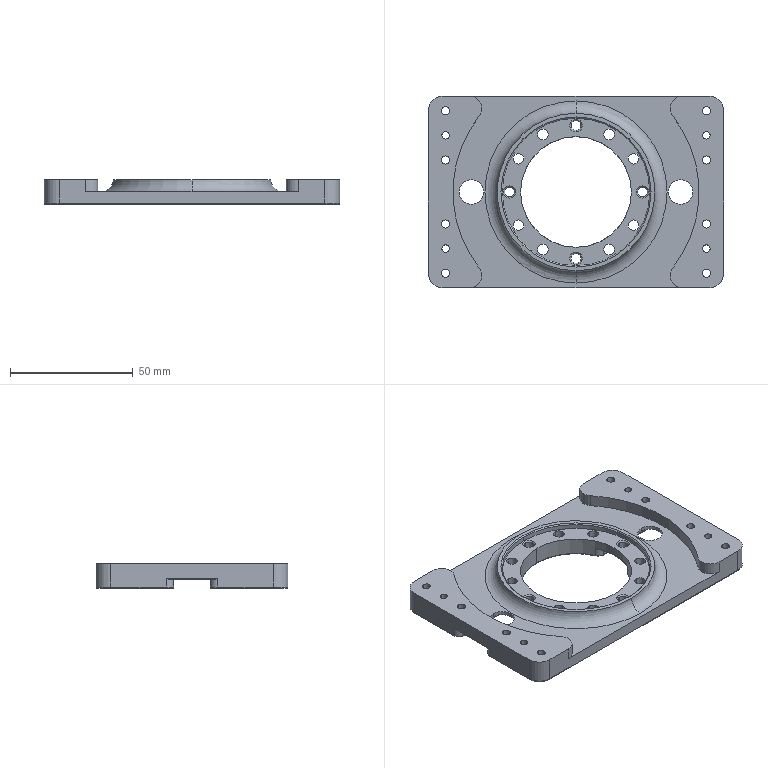NC program | NX | posted with a generic post | part box 120 x 78 x 10 mm
Lines 35 to 888 of 8419:
(ADAPTIVE_MILLING_COPY_1 , TOOL : D10)
N68 T15 M6
N70 G54
N72 G17 G0 G90 X-29.216 Y42.583 B0. C0. S9500 M3
N74 G43 Z30. H15
N76 Z3.
N78 G94 G3 X-29.216 Y42.583 Z2.506 I1.305 J-4.307 F1000.
N80 X-29.216 Y42.583 Z2.013 I1.305 J-4.307
N82 X-29.216 Y42.583 Z1.519 I1.305 J-4.307
N84 X-29.216 Y42.583 Z1.026 I1.305 J-4.307
N86 X-29.216 Y42.583 Z0.532 I1.305 J-4.307
N88 X-29.216 Y42.583 Z0.039 I1.305 J-4.307
N90 X-29.216 Y42.583 Z-0.455 I1.305 J-4.307
N92 X-29.216 Y42.583 Z-0.948 I1.305 J-4.307
N94 X-29.216 Y42.583 Z-1.442 I1.305 J-4.307
N96 X-29.216 Y42.583 Z-1.935 I1.305 J-4.307
N98 X-29.216 Y42.583 Z-2.429 I1.305 J-4.307
N100 X-29.216 Y42.583 Z-2.922 I1.305 J-4.307
N102 X-29.216 Y42.583 Z-3.416 I1.305 J-4.307
N104 X-29.216 Y42.583 Z-3.909 I1.305 J-4.307
N106 X-29.216 Y42.583 Z-4.403 I1.305 J-4.307
N108 X-23.412 Y38.276 Z-4.75 R-4.5
N110 X-24.233 Y35.67 R-4.501 F3000.
N112 X-28.904 Y43.148 R4.673
N114 X-24.107 Y35.033 R-4.978
N116 X-29.565 Y43.485 R5.194
N118 X-24.488 Y33.987 R-5.474
N120 X-22.23 Y38.968 R5.736
N122 X-26.259 Y44. R5.522
N124 X-29.504 Y43.925 R23.784
N126 X-33.902 Y37.98 R5.67
N128 X-33.017 Y35.334 R42.36
N130 X-25.859 Y32.634 R5.739
N132 G2 X-23.479 Y34.38 R62.429
N134 G3 X-23.21 Y42.728 R5.954
N136 X-24.77 Y43.953 R4.725
N138 X-26.263 Y44. R8.377
N140 G1 X-28.759
N142 G3 X-30.982 Y43.785 R5.996
N144 X-34.405 Y39.201 R5.651
N146 X-33.91 Y38.004 R3.106
N148 G1 X-33.87 Y37.886
N150 G3 X-31.896 Y37.646 R1.101
N152 G1 X-28.953 Y42.313
N154 G3 X-29.884 Y44. R1.102
N156 X-33.692 Y42.286 R4.141
N158 X-34.785 Y39.935 R4.907
N160 G1 X-34.689 Y39.448
N162 X-34.269 Y38.68
N164 G3 X-32.399 Y38.583 R1.102
N166 G1 X-29.853 Y42.276
N168 G3 X-30.759 Y44. R1.101
N170 X-34.15 Y42.492 R3.819
N172 X-35.125 Y40.375 R3.599
N174 X-34.774 Y39.604 R1.466
N176 G1 X-34.654 Y39.385
N178 G3 X-32.801 Y39.264 R1.102
N180 G1 X-30.62 Y42.252
N182 G3 X-31.509 Y44. R1.101
N184 X-34.832 Y42.382 R3.64
N186 X-35.433 Y40.652 R2.554
N188 X-34.862 Y39.726 R2.225
N190 X-33.128 Y39.755 R1.103
N192 G1 X-31.256 Y42.238
N194 G3 X-32.134 Y44. R1.101
N196 X-35.752 Y41.266 R3.309
N198 X-35.244 Y40.198 R1.572
N200 X-33.507 Y40.231 R1.103
N202 G1 X-32.003 Y42.241
N204 G3 X-32.884 Y44. R1.101
N206 X-36.031 Y41.587 R2.885
N208 X-35.525 Y40.547 R1.585
N210 X-33.8 Y40.565 R1.103
N212 G1 X-32.514 Y42.227
N214 G3 X-33.384 Y44. R1.101
N216 X-36.282 Y41.996 R2.631
N218 X-35.832 Y40.927 R1.303
N220 X-34.098 Y40.955 R1.103
N222 G1 X-33.131 Y42.237
N224 G3 X-34.009 Y44. R1.101
N226 X-36.533 Y42.113 R2.243
N228 X-35.977 Y41.092 R1.23
N230 X-34.386 Y41.255 R1.104
N232 G1 X-33.954 Y41.808
N234 X-33.541 Y42.376
N236 G3 X-34.509 Y44. R1.102
N238 X-36.761 Y42.197 R1.959
N240 X-36.163 Y41.253 R1.343
N242 X-33.477 Y42.652 R1.627
N244 X-35.009 Y44. R1.549
N246 X-36.951 Y42.244 R1.668
N248 X-36.37 Y41.432 R1.432
N250 X-34.796 Y43.876 R-1.469
N252 G1 X-35.084 Y43.965
N254 X-35.384 Y44.
N256 G3 X-37.134 Y42.387 R1.49
N258 X-36.65 Y41.673 R1.326
N260 X-35.371 Y43.942 R-1.33
N262 G1 X-35.563 Y43.981
N264 X-35.759 Y44.
N266 G3 X-37.254 Y42.381 R1.299
N268 X-36.805 Y41.807 R1.541
N270 X-34.871 Y42.896 R1.185
N272 X-36.134 Y44. R1.28
N274 X-36.954 Y41.935 R1.14
N276 X-35.171 Y42.832 R1.085
N278 X-36.384 Y44. R1.218
N280 X-37.089 Y42.051 R1.073
N282 G1 X-35.91 Y41.024
N284 X-34.774 Y39.604
N286 X-33.91 Y38.004
N288 X-33.345 Y36.276
N290 G3 X-30.887 Y32.471 R4.45
N292 X-26.905 Y31.809 R5.657
N294 X-25.718 Y32.727 R7.011
N296 X-26.059 Y34.611 R1.102
N298 G1 X-31.77 Y36.603
N300 G3 X-33.222 Y35.41 R1.102
N302 X-31.163 Y32.059 R4.006
N304 X-27.713 Y31.192 R5.311
N306 X-26.602 Y31.991 R3.861
N308 X-26.912 Y33.864 R1.102
N310 G1 X-31.61 Y35.664
N312 G3 X-33.101 Y34.559 R1.102
N314 X-31.961 Y32.097 R3.055
N316 X-28.454 Y30.672 R5.173
N318 X-27.959 Y30.862 R4.213
N320 G1 X-27.287 Y31.422
N322 G3 X-27.512 Y33.258 R1.102
N324 G1 X-31.529 Y35.196
N326 G3 X-33.106 Y34.248 R1.102
N328 X-31.927 Y31.494 R3.116
N330 X-28.881 Y30.25 R4.319
N332 X-28.072 Y30.768 R1.522
N334 G1 X-27.88 Y30.928
N336 G3 X-28.045 Y32.733 R1.102
N338 G1 X-31.487 Y34.665
N340 G3 X-33.125 Y33.748 R1.102
N342 X-31.896 Y30.892 R3.172
N344 X-29.292 Y29.854 R3.731
N346 X-28.289 Y30.554 R1.904
N348 X-28.481 Y32.262 R1.103
N350 G1 X-31.459 Y34.137
N352 G3 X-33.144 Y33.249 R1.102
N354 X-31.761 Y30.224 R3.197
N356 X-29.565 Y29.502 R2.968
N358 X-28.667 Y30.175 R2.079
N360 X-28.858 Y31.882 R1.103
N362 G1 X-31.485 Y33.541
N364 G3 X-33.163 Y32.752 R1.102
N366 X-32.408 Y30.263 R2.636
N368 X-29.997 Y29.139 R3.094
N370 X-29.091 Y29.75 R1.694
N372 X-29.226 Y31.419 R1.103
N374 G1 X-31.512 Y33.068
N376 G3 X-33.229 Y32.414 R1.102
N378 X-32.48 Y29.785 R2.614
N380 X-30.268 Y28.824 R2.713
N382 X-29.424 Y29.416 R1.751
N384 X-29.518 Y31.054 R1.103
N386 G1 X-31.552 Y32.671
N388 G3 X-33.31 Y32.047 R1.102
N390 X-32.356 Y29.15 R2.639
N392 X-30.524 Y28.527 R2.255
N394 X-29.73 Y29.11 R1.862
N396 X-29.831 Y30.753 R1.103
N398 G1 X-31.667 Y32.188
N400 G3 X-33.418 Y31.559 R1.102
N402 X-32.391 Y28.703 R2.551
N404 X-30.762 Y28.252 R1.928
N406 X-30.023 Y28.817 R2.004
N408 X-30.141 Y30.473 R1.103
N410 G1 X-31.792 Y31.713
N412 G3 X-33.526 Y31.071 R1.102
N414 X-32.839 Y28.626 R2.276
N416 X-31.041 Y27.975 R1.936
N418 X-30.297 Y28.542 R1.994
N420 X-30.406 Y30.191 R1.103
N422 G1 X-31.893 Y31.331
N424 G3 X-33.576 Y30.884 R1.103
N426 X-33.225 Y28.559 R2.073
N428 X-31.393 Y27.685 R2.031
N430 X-30.615 Y28.223 R1.624
N432 X-30.683 Y29.839 R1.104
N434 G1 X-31.996 Y30.952
N436 G3 X-33.722 Y30.538 R1.103
N438 X-33.185 Y28.035 R2.108
N440 X-31.491 Y27.463 R1.759
N442 X-30.825 Y28.009 R1.548
N444 X-30.939 Y29.531 R1.104
N446 G1 X-32.119 Y30.587
N448 G3 X-33.867 Y30.192 R1.102
N450 X-33.298 Y27.705 R2.059
N452 X-31.584 Y27.258 R1.615
N454 X-31.021 Y27.773 R1.922
N456 X-31.162 Y29.318 R1.104
N458 G1 X-31.788 Y29.851
N460 X-32.43 Y30.364
N462 G3 X-34.012 Y29.847 R1.103
N464 X-33.298 Y27.303 R2.026
N466 X-31.57 Y27.147 R1.399
N468 G1 X-31.465 Y27.237
N470 X-31.226 Y27.526
N472 G3 X-31.318 Y29.028 R1.104
N474 G1 X-31.889 Y29.575
N476 X-32.477 Y30.101
N478 G3 X-34.108 Y29.616 R1.103
N480 X-33.504 Y27.077 R1.979
N482 X-31.78 Y26.897 R1.387
N484 G1 X-31.685 Y26.977
N486 X-31.666 Y26.994
N488 X-31.427 Y27.283
N490 G3 X-31.588 Y28.845 R1.104
N492 G1 X-32.152 Y29.301
N494 X-32.731 Y29.738
N496 G3 X-34.243 Y29.294 R1.104
N498 X-33.985 Y27.134 R1.759
N500 X-32.218 Y26.517 R1.589
N502 X-31.622 Y27.048 R1.784
N504 X-31.79 Y28.616 R1.104
N506 G1 X-32.341 Y29.054
N508 X-32.908 Y29.472
N510 G3 X-34.356 Y29.106 R1.106
N512 X-34.176 Y26.916 R1.749
N514 X-32.418 Y26.281 R1.581
N516 X-31.814 Y26.816 R1.765
N518 X-31.946 Y28.353 R1.104
N520 G1 X-32.462 Y28.801
N522 X-32.992 Y29.232
N524 G3 X-34.492 Y28.896 R1.104
N526 X-34.287 Y26.608 R1.768
N528 X-32.617 Y26.049 R1.538
N530 X-32.002 Y26.589 R1.737
N532 X-32.101 Y28.097 R1.104
N534 G1 X-32.59 Y28.557
N536 X-33.094 Y29.001
N538 G3 X-34.629 Y28.687 R1.104
N540 X-34.391 Y26.306 R1.771
N542 X-32.702 Y25.872 R1.442
N544 X-32.188 Y26.365 R2.331
N546 X-32.345 Y27.923 R1.104
N548 G1 X-32.846 Y28.331
N550 X-33.359 Y28.724
N552 G3 X-34.833 Y28.372 R1.104
N554 X-34.581 Y26.094 R1.741
N556 X-32.896 Y25.643 R1.44
N558 X-32.371 Y26.144 R2.289
N560 X-32.498 Y27.677 R1.104
N562 G1 X-32.975 Y28.094
N564 X-33.465 Y28.496
N566 G3 X-34.969 Y28.163 R1.104
N568 X-34.766 Y25.886 R1.715
N570 X-33.087 Y25.419 R1.432
N572 X-32.552 Y25.926 R2.257
N574 X-32.751 Y27.517 R1.104
N576 G1 X-33.247 Y27.883
N578 X-33.756 Y28.231
N580 G3 X-35.174 Y27.848 R1.106
N582 X-34.922 Y25.651 R1.697
N584 X-33.239 Y25.217 R1.406
N586 X-32.737 Y25.702 R2.399
N588 X-32.868 Y27.239 R1.104
N590 G1 X-33.325 Y27.637
N592 X-33.798 Y28.016
N594 G3 X-35.261 Y27.716 R1.106
N596 X-35.107 Y25.446 R1.675
N598 X-33.321 Y25.061 R1.374
N600 G1 X-32.914 Y25.489
N602 G3 X-33.022 Y27.006 R1.104
N604 G1 X-33.458 Y27.405
N606 X-33.907 Y27.79
N608 G3 X-35.406 Y27.512 R1.104
N610 X-35.291 Y25.241 R1.673
N612 X-33.616 Y24.773 R1.41
N614 X-33.09 Y25.276 R2.26
N616 X-33.282 Y26.862 R1.104
N618 G1 X-33.747 Y27.211
N620 X-34.224 Y27.543
N622 G3 X-35.625 Y27.208 R1.106
N624 X-35.468 Y25.036 R1.655
N626 X-33.797 Y24.539 R1.436
N628 X-33.279 Y25.045 R1.538
N630 X-33.404 Y26.438 R1.106
N632 G1 X-33.808 Y26.851
N634 X-34.225 Y27.25
N636 G3 X-35.771 Y27.005 R1.104
N638 X-35.565 Y24.741 R1.665
N640 X-33.871 Y24.359 R1.397
N642 X-33.364 Y24.921 R1.951
N644 X-33.572 Y26.39 R1.106
N646 G1 X-34.014 Y26.76
N648 X-34.47 Y27.112
N650 G3 X-35.916 Y26.801 R1.106
N652 X-35.742 Y24.537 R1.657
N654 X-33.946 Y24.188 R1.384
N656 X-33.515 Y24.698 R2.672
N658 X-33.708 Y26.154 R1.106
N660 G1 X-34.146 Y26.536
N662 X-34.599 Y26.899
N664 G3 X-36.062 Y26.598 R1.106
N666 X-35.916 Y24.333 R1.651
N668 X-34.124 Y23.947 R1.403
N670 X-33.666 Y24.478 R2.38
N672 X-33.955 Y26.008 R1.104
N674 G1 X-34.429 Y26.335
N676 X-34.914 Y26.646
N678 G3 X-36.28 Y26.293 R1.106
N680 X-36.094 Y24.128 R1.639
N682 X-34.413 Y23.642 R1.469
N684 X-33.815 Y24.26 R1.675
N686 X-34.09 Y25.78 R1.104
N688 G1 X-34.563 Y26.116
N690 X-35.047 Y26.436
N692 G3 X-36.426 Y26.09 R1.106
N694 X-36.27 Y23.923 R1.634
N696 X-34.595 Y23.402 R1.495
N698 X-33.978 Y24.022 R1.593
N700 X-34.219 Y25.517 R1.104
N702 G1 X-34.682 Y25.875
N704 X-35.158 Y26.216
N706 G3 X-36.572 Y25.887 R1.106
N708 X-36.362 Y23.625 R1.662
N710 X-34.667 Y23.216 R1.432
N712 X-34.135 Y23.792 R1.829
N714 X-34.352 Y25.269 R1.106
N716 G1 X-34.809 Y25.643
N718 X-35.28 Y26.
N720 G3 X-36.717 Y25.684 R1.106
N722 X-36.542 Y23.419 R1.661
N724 X-34.745 Y23.038 R1.415
N726 X-34.286 Y23.57 R2.373
N728 X-34.488 Y25.034 R1.106
N730 G1 X-34.942 Y25.42
N732 X-35.41 Y25.787
N734 G3 X-36.863 Y25.481 R1.106
N736 X-36.721 Y23.214 R1.661
N738 X-34.928 Y22.793 R1.438
N740 X-34.437 Y23.35 R2.218
N742 X-34.733 Y24.885 R1.104
N744 G1 X-35.223 Y25.216
N746 X-35.723 Y25.532
N748 G3 X-37.082 Y25.176 R1.106
N750 X-36.983 Y23.103 R1.623
N752 X-35.224 Y22.487 R1.545
N754 X-34.601 Y23.11 R1.581
N756 X-34.861 Y24.619 R1.104
N758 G1 X-35.341 Y24.974
N760 X-35.832 Y25.311
N762 G3 X-37.227 Y24.973 R1.106
N764 X-37.081 Y22.802 R1.647
N766 X-35.41 Y22.245 R1.54
N768 X-34.758 Y22.881 R1.535
N770 X-34.994 Y24.372 R1.104
N772 G1 X-35.468 Y24.743
N774 X-35.955 Y25.096
N776 G3 X-37.373 Y24.77 R1.106
N778 X-37.228 Y22.559 R1.658
N780 X-35.552 Y22.021 R1.529
N782 X-34.916 Y22.649 R1.558
N784 X-35.169 Y24.154 R1.104
N786 G1 X-35.651 Y24.516
N788 X-36.146 Y24.861
N790 G3 X-37.547 Y24.526 R1.106
N792 X-37.147 Y22.108 R1.736
N794 X-35.279 Y22.118 R1.296
N796 G1 X-35.067 Y22.428
N798 G3 X-35.301 Y23.917 R1.104
N800 G1 X-35.767 Y24.284
N802 X-36.246 Y24.635
N804 G3 X-37.726 Y24.232 R1.104
N806 X-37.317 Y21.892 R1.704
N808 X-35.509 Y21.81 R1.313
N810 G1 X-35.425 Y21.903
N812 X-35.211 Y22.217
N814 G3 X-35.552 Y23.781 R1.104
N816 G1 X-36.05 Y24.084
N818 X-36.557 Y24.37
N820 G3 X-37.917 Y23.909 R1.106
N822 X-37.478 Y21.673 R1.685
N824 X-35.669 Y21.564 R1.324
N826 G1 X-35.584 Y21.656
N828 X-35.513 Y21.749
N830 X-35.448 Y21.866
N832 X-35.423 Y21.908
N834 G3 X-35.632 Y23.312 R1.106
N836 G1 X-36.065 Y23.697
N838 X-36.511 Y24.066
N840 G3 X-38.044 Y23.693 R1.104
N842 X-37.643 Y21.454 R1.672
N844 X-35.826 Y21.304 R1.357
N846 X-35.467 Y21.833 R3.346
N848 X-35.801 Y23.27 R1.106
N850 G1 X-36.27 Y23.601
N852 X-36.752 Y23.913
N854 G3 X-38.171 Y23.478 R1.106
N856 X-37.802 Y21.235 R1.669
N858 X-36.08 Y20.971 R1.424
N860 X-35.597 Y21.598 R1.805
N862 X-35.915 Y23.024 R1.106
N864 G1 X-36.382 Y23.367
N866 X-36.863 Y23.69
N868 G3 X-38.298 Y23.263 R1.106
N870 X-37.861 Y20.939 R1.669
N872 X-36.045 Y20.875 R1.343
N874 G1 X-35.726 Y21.367
N876 G3 X-36.149 Y22.86 R1.104
N878 G1 X-36.648 Y23.144
N880 X-37.157 Y23.412
N882 G3 X-38.488 Y22.94 R1.106
N884 X-38.116 Y20.799 R1.638
N886 X-36.296 Y20.532 R1.429
N888 X-35.856 Y21.132 R2.134
N890 X-36.261 Y22.614 R1.104
N892 G1 X-36.758 Y22.91
N894 X-37.266 Y23.189
N896 G3 X-38.615 Y22.725 R1.106
N898 X-38.277 Y20.579 R1.634
N900 X-36.455 Y20.274 R1.462
N902 X-35.993 Y20.886 R1.903
N904 X-36.368 Y22.35 R1.104
N906 G1 X-36.86 Y22.665
N908 X-37.364 Y22.962
N910 G3 X-38.743 Y22.509 R1.106
N912 X-38.34 Y20.277 R1.647
N914 X-36.614 Y20.015 R1.444
N916 X-36.126 Y20.646 R1.788
N918 X-36.479 Y22.096 R1.106
N920 G1 X-36.968 Y22.426
N922 X-37.469 Y22.737
N924 G3 X-38.87 Y22.294 R1.106
N926 X-38.499 Y20.058 R1.64
N928 X-36.776 Y19.755 R1.467
N930 X-36.257 Y20.411 R1.706
N932 X-36.593 Y21.849 R1.106
N934 G1 X-37.08 Y22.191
N936 X-37.58 Y22.514
N938 G3 X-38.997 Y22.079 R1.106
N940 X-38.656 Y19.836 R1.65
N942 X-36.936 Y19.498 R1.487
N944 X-36.393 Y20.166 R1.634
N946 X-36.817 Y21.66 R1.104
N948 G1 X-37.332 Y21.953
N950 X-37.857 Y22.228
N952 G3 X-39.187 Y21.756 R1.106
N954 X-38.906 Y19.702 R1.615
N956 X-37.101 Y19.238 R1.55
N958 X-36.53 Y19.919 R1.566
N960 X-36.923 Y21.395 R1.104
N962 G1 X-37.433 Y21.707
N964 X-37.954 Y22.001
N966 G3 X-39.314 Y21.54 R1.106
N968 X-38.979 Y19.391 R1.649
N970 X-37.266 Y18.979 R1.549
N972 X-36.664 Y19.678 R1.522
N974 X-37.034 Y21.14 R1.104
N976 G1 X-37.54 Y21.467
N978 X-38.058 Y21.776
N980 G3 X-39.441 Y21.325 R1.106
N982 X-39.059 Y19.096 R1.667
N984 X-37.232 Y18.844 R1.451
N986 X-36.794 Y19.444 R2.174
N988 X-37.203 Y20.93 R1.104
N990 G1 X-37.724 Y21.237
N992 X-38.256 Y21.525
N994 G3 X-39.62 Y21.014 R1.106
N996 X-39.015 Y18.713 R1.72
N998 X-37.201 Y18.758 R1.332
N1000 G1 X-37.116 Y18.865
N1002 X-36.934 Y19.193
N1004 G3 X-37.378 Y20.698 R1.104
N1006 G1 X-37.901 Y20.981
N1008 X-38.434 Y21.244
N1010 G3 X-39.781 Y20.675 R1.106
N1012 X-39.163 Y18.48 R1.695
N1014 X-37.346 Y18.504 R1.339
N1016 G1 X-37.267 Y18.6
N1018 X-37.251 Y18.622
N1020 X-37.069 Y18.95
N1022 G3 X-37.486 Y20.44 R1.104
N1024 G1 X-37.995 Y20.734
N1026 X-38.515 Y21.009
N1028 G3 X-39.889 Y20.45 R1.106
N1030 X-39.307 Y18.25 R1.672
N1032 X-37.578 Y18.161 R1.373
N1034 X-37.232 Y18.655 R3.054
N1036 X-37.566 Y20.092 R1.106
N1038 G1 X-38.04 Y20.425
N1040 X-38.525 Y20.742
N1042 G3 X-39.996 Y20.224 R1.104
N1044 X-39.452 Y18.019 R1.658
N1046 X-37.624 Y17.978 R1.378
N1048 X-37.334 Y18.459 R2.923
N1050 X-37.76 Y19.834 R1.106
N1052 G1 X-38.241 Y20.137
N1054 X-38.732 Y20.424
N1056 G3 X-40.157 Y19.885 R1.104
N1058 X-39.589 Y17.788 R1.638
N1060 X-37.85 Y17.626 R1.447
N1062 X-37.388 Y18.335 R1.69
N1064 X-37.928 Y19.771 R1.104
N1066 G1 X-38.443 Y20.016
N1068 X-38.965 Y20.243
N1070 G3 X-40.265 Y19.66 R1.106
N1072 X-39.625 Y17.483 R1.649
N1074 X-37.802 Y17.524 R1.362
N1076 X-37.5 Y18.078 R3.781
N1078 X-38.01 Y19.499 R1.104
N1080 G1 X-38.522 Y19.763
N1082 X-39.043 Y20.008
N1084 G3 X-40.372 Y19.434 R1.106
N1086 X-39.862 Y17.324 R1.63
N1088 X-38.024 Y17.164 R1.454
N1090 X-37.61 Y17.826 R1.842
N1092 X-38.096 Y19.236 R1.106
N1094 G1 X-38.607 Y19.515
N1096 X-39.128 Y19.775
N1098 G3 X-40.48 Y19.208 R1.106
N1100 X-40.001 Y17.092 R1.626
N1102 X-38.16 Y16.892 R1.484
N1104 X-37.718 Y17.581 R1.737
N1106 X-38.187 Y18.981 R1.106
N1108 G1 X-38.697 Y19.272
N1110 X-39.219 Y19.544
N1112 G3 X-40.587 Y18.982 R1.106
N1114 X-40.042 Y16.782 R1.645
N1116 X-38.203 Y16.7 R1.436
N1118 X-37.824 Y17.339 R2.217
N1120 X-38.403 Y18.793 R1.104
N1122 G1 X-38.941 Y19.024
N1124 X-39.485 Y19.237
N1126 G3 X-40.748 Y18.644 R1.106
N1128 X-40.181 Y16.547 R1.635
N1130 X-38.436 Y16.346 R1.509
N1132 X-37.94 Y17.073 R1.583
N1134 X-38.479 Y18.509 R1.104
N1136 G1 X-39.013 Y18.765
N1138 X-39.555 Y19.001
N1140 G3 X-40.856 Y18.418 R1.106
N1142 X-40.321 Y16.313 R1.632
N1144 X-38.477 Y16.146 R1.485
N1146 X-38.051 Y16.819 R1.792
N1148 X-38.564 Y18.242 R1.104
N1150 G1 X-39.096 Y18.515
N1152 X-39.637 Y18.768
N1154 G3 X-40.963 Y18.192 R1.106
N1156 X-40.458 Y16.08 R1.631
N1158 X-38.613 Y15.873 R1.507
N1160 X-38.159 Y16.574 R1.707
N1162 X-38.654 Y17.988 R1.104
N1164 G1 X-39.186 Y18.272
N1166 X-39.728 Y18.537
N1168 G3 X-41.071 Y17.967 R1.106
N1170 X-40.5 Y15.769 R1.655
N1172 X-38.753 Y15.596 R1.507
N1174 X-38.273 Y16.313 R1.622
N1176 X-38.737 Y17.711 R1.106
N1178 G1 X-39.265 Y18.016
N1180 X-39.805 Y18.301
N1182 G3 X-41.178 Y17.741 R1.106
N1184 X-40.651 Y15.545 R1.653
N1186 X-38.806 Y15.386 R1.483
N1188 X-38.385 Y16.055 R1.81
N1190 X-38.949 Y17.503 R1.104
N1192 G1 X-39.502 Y17.752
N1194 X-40.065 Y17.98
N1196 G3 X-41.372 Y17.298 R1.106
N1198 X-40.574 Y15.157 R1.709
N1200 X-38.757 Y15.298 R1.36
N1202 G1 X-38.683 Y15.4
N1204 X-38.645 Y15.462
N1206 X-38.495 Y15.805
N1208 G3 X-39.035 Y17.242 R1.104
N1210 G1 X-39.578 Y17.502
N1212 X-40.13 Y17.74
N1214 G3 X-41.459 Y17.064 R1.106
N1216 X-40.592 Y14.85 R1.714
N1218 X-38.755 Y15.21 R1.299
N1220 G1 X-38.605 Y15.554
N1222 G3 X-39.12 Y16.978 R1.104
N1224 G1 X-39.645 Y17.244
N1226 X-40.177 Y17.493
N1228 G3 X-41.546 Y16.829 R1.104
N1230 X-40.825 Y14.671 R1.674
N1232 X-39.088 Y14.67 R1.402
N1234 X-38.715 Y15.303 R2.261
N1236 X-39.332 Y16.773 R1.104
N1238 G1 X-39.873 Y16.982
N1240 X-40.421 Y17.172
N1242 G3 X-41.677 Y16.478 R1.106
N1244 X-40.842 Y14.361 R1.674
N1246 X-39.044 Y14.593 R1.324
N1248 G1 X-38.977 Y14.699
N1250 X-38.937 Y14.782
N1252 X-38.928 Y14.81
N1254 X-38.909 Y14.858
N1256 X-38.859 Y14.973
N1258 G3 X-39.362 Y16.391 R1.104
N1260 G1 X-39.869 Y16.656
N1262 X-40.383 Y16.904
N1264 G3 X-41.764 Y16.243 R1.104
N1266 X-40.961 Y14.117 R1.668
N1268 X-39.151 Y14.31 R1.349
N1270 X-38.928 Y14.81 R4.372
N1272 X-39.435 Y16.111 R1.106
N1274 G1 X-39.932 Y16.393
N1276 X-40.438 Y16.658
N1278 G3 X-41.851 Y16.009 R1.104
N1280 X-41.079 Y13.874 R1.652
N1282 X-39.257 Y14.025 R1.376
N1284 X-38.983 Y14.641 R2.591
N1286 X-39.564 Y15.98 R1.106
N1288 G1 X-40.083 Y16.226
N1290 X-40.612 Y16.452
N1292 G3 X-41.938 Y15.775 R1.106
N1294 X-41.089 Y13.568 R1.668
N1296 X-39.29 Y13.838 R1.344
N1298 G1 X-39.064 Y14.392
N1300 G3 X-39.765 Y15.778 R1.104
N1302 G1 X-40.307 Y15.96
N1304 X-40.855 Y16.125
N1306 G3 X-42.068 Y15.423 R1.106
N1308 X-41.312 Y13.387 R1.634
N1310 X-39.473 Y13.454 R1.432
N1312 X-39.151 Y14.127 R2.022
N1314 X-39.821 Y15.503 R1.104
N1316 G1 X-40.364 Y15.704
N1318 X-40.914 Y15.886
N1320 G3 X-42.155 Y15.189 R1.106
N1322 X-41.429 Y13.142 R1.632
N1324 X-39.582 Y13.167 R1.459
N1326 X-39.237 Y13.864 R1.852
N1328 X-39.879 Y15.229 R1.104
N1330 G1 X-40.423 Y15.447
N1332 X-40.975 Y15.646
N1334 G3 X-42.242 Y14.954 R1.106
N1336 X-41.439 Y12.83 R1.657
N1338 X-39.692 Y12.882 R1.456
N1340 X-39.32 Y13.608 R1.741
N1342 X-39.944 Y14.966 R1.106
N1344 G1 X-40.49 Y15.197
N1346 X-41.044 Y15.407
N1348 G3 X-42.329 Y14.72 R1.106
N1350 X-41.554 Y12.586 R1.657
N1352 X-39.716 Y12.686 R1.433
N1354 X-39.402 Y13.357 R2.243
N1356 X-40.012 Y14.709 R1.106
N1358 G1 X-40.561 Y14.95
N1360 X-41.118 Y15.17
N1362 G3 X-42.416 Y14.486 R1.106
N1364 X-41.673 Y12.341 R1.653
N1366 X-39.917 Y12.307 R1.507
N1368 X-39.493 Y13.079 R1.582
N1370 X-40.186 Y14.462 R1.104
N1372 G1 X-40.753 Y14.658
N1374 X-41.326 Y14.835
N1376 G3 X-42.547 Y14.134 R1.106
N1378 X-41.894 Y12.164 R1.625
N1380 X-40.031 Y12.022 R1.575
N1382 X-39.579 Y12.817 R1.53
N1384 X-40.246 Y14.192 R1.104
N1386 G1 X-40.815 Y14.404
N1388 X-41.39 Y14.596
N1390 G3 X-42.633 Y13.9 R1.106
N1392 X-41.706 Y11.728 R1.698
N1394 X-39.974 Y11.895 R1.413
N1396 X-39.661 Y12.566 R2.241
N1398 X-40.325 Y13.939 R1.104
N1400 G1 X-40.897 Y14.156
N1402 X-41.477 Y14.349
N1404 G3 X-42.744 Y13.558 R1.106
N1406 X-41.813 Y11.475 R1.702
N1408 X-40.077 Y11.613 R1.426
N1410 X-39.751 Y12.29 R1.986
N1412 X-40.374 Y13.648 R1.106
N1414 G1 X-40.927 Y13.881
N1416 X-41.488 Y14.096
N1418 G3 X-42.81 Y13.317 R1.104
N1420 X-41.807 Y11.165 R1.707
N1422 X-40.027 Y11.533 R1.341
N1424 G1 X-39.967 Y11.642
N1426 X-39.954 Y11.669
N1428 X-39.838 Y12.025
N1430 G3 X-40.557 Y13.417 R1.104
N1432 G1 X-41.122 Y13.597
N1434 X-41.694 Y13.755
N1436 G3 X-42.908 Y12.955 R1.106
N1438 X-41.906 Y10.91 R1.682
N1440 X-40.121 Y11.255 R1.344
N1442 G1 X-40.06 Y11.365
N1444 X-40.041 Y11.404
N1446 X-39.924 Y11.76
N1448 G3 X-40.614 Y13.143 R1.104
N1450 G1 X-41.169 Y13.337
N1452 X-41.731 Y13.509
N1454 G3 X-42.974 Y12.714 R1.106
N1456 X-42.006 Y10.657 R1.669
N1458 X-40.215 Y10.98 R1.349
N1460 G1 X-40.153 Y11.089
N1462 X-40.126 Y11.144
N1464 X-40.009 Y11.5
N1466 G3 X-40.674 Y12.874 R1.104
N1468 G1 X-41.22 Y13.08
N1470 X-41.774 Y13.264
N1472 G3 X-43.04 Y12.473 R1.106
N1474 X-42.102 Y10.403 R1.664
N1476 X-40.38 Y10.605 R1.385
N1478 X-40.123 Y11.15 R2.652
N1480 X-40.666 Y12.47 R1.106
N1482 G1 X-41.181 Y12.739
N1484 X-41.706 Y12.989
N1486 G3 X-43.106 Y12.232 R1.104
N1488 X-42.084 Y10.096 R1.681
N1490 X-40.322 Y10.522 R1.324
N1492 G1 X-40.268 Y10.635
N1494 X-40.232 Y10.73
N1496 X-40.178 Y10.974
N1498 G3 X-40.833 Y12.231 R1.106
N1500 G1 X-41.356 Y12.449
N1502 X-41.886 Y12.65
N1504 G3 X-43.205 Y11.87 R1.104
N1506 X-42.293 Y9.899 R1.635
N1508 X-40.469 Y10.123 R1.417
N1510 X-40.21 Y10.828 R1.982
N1512 X-40.974 Y12.123 R1.104
N1514 G1 X-41.52 Y12.287
N1516 X-42.071 Y12.43
N1518 G3 X-43.271 Y11.629 R1.106
N1520 X-42.276 Y9.59 R1.65
N1522 X-40.552 Y9.828 R1.417
N1524 X-40.269 Y10.563 R1.818
N1526 X-41.01 Y11.851 R1.106
N1528 G1 X-41.56 Y12.029
N1530 X-42.115 Y12.186
N1532 G3 X-43.337 Y11.388 R1.106
N1534 X-42.37 Y9.337 R1.643
N1536 X-40.559 Y9.633 R1.406
N1538 X-40.327 Y10.305 R2.336
N1540 X-41.053 Y11.588 R1.106
N1542 G1 X-41.607 Y11.776
N1544 X-42.168 Y11.943
N1546 G3 X-43.402 Y11.147 R1.106
N1548 X-42.464 Y9.083 R1.642
N1550 X-40.64 Y9.335 R1.432
N1552 X-40.387 Y10.034 R2.046
N1554 X-41.218 Y11.346 R1.104
N1556 G1 X-41.788 Y11.478
N1558 X-42.363 Y11.592
N1560 G3 X-43.501 Y10.785 R1.106
N1562 X-42.666 Y8.888 R1.614
N1564 X-40.804 Y8.946 R1.539
N1566 X-40.447 Y9.765 R1.559
N1568 X-41.25 Y11.07 R1.104
N1570 G1 X-41.824 Y11.219
N1572 X-42.403 Y11.349
N1574 G3 X-43.567 Y10.544 R1.106
N1576 X-42.65 Y8.573 R1.636
N1578 X-40.805 Y8.741 R1.487
N1580 X-40.506 Y9.499 R1.746
N1582 X-41.286 Y10.798 R1.104
N1584 G1 X-41.864 Y10.962
N1586 X-42.448 Y11.106
N1588 G3 X-43.633 Y10.303 R1.106
N1590 X-42.747 Y8.319 R1.637
N1592 X-40.892 Y8.441 R1.522
N1594 X-40.564 Y9.238 R1.661
N1596 X-41.327 Y10.533 R1.104
N1598 G1 X-41.91 Y10.708
N1600 X-42.498 Y10.863
N1602 G3 X-43.699 Y10.061 R1.106
N1604 X-42.628 Y7.957 R1.698
N1606 X-40.903 Y8.229 R1.448
N1608 X-40.627 Y8.955 R1.857
N1610 X-41.361 Y10.24 R1.106
N1612 G1 X-41.938 Y10.431
N1614 X-42.521 Y10.603
N1616 G3 X-43.778 Y9.712 R1.104
N1618 X-42.595 Y7.649 R1.719
N1620 X-40.906 Y8.035 R1.381
N1622 X-40.688 Y8.682 R2.514
N1624 X-41.518 Y9.994 R1.104
N1626 G1 X-42.104 Y10.131
N1628 X-42.694 Y10.246
N1630 G3 X-43.845 Y9.343 R1.106
N1632 X-42.676 Y7.386 R1.687
N1634 X-40.978 Y7.748 R1.398
N1636 X-40.747 Y8.417 R2.346
N1638 X-41.554 Y9.724 R1.104
N1640 G1 X-42.133 Y9.872
N1642 X-42.717 Y9.999
N1644 G3 X-43.889 Y9.097 R1.106
N1646 X-42.753 Y7.123 R1.681
N1648 X-41.049 Y7.461 R1.402
N1650 X-40.806 Y8.151 R2.272
N1652 X-41.589 Y9.451 R1.104
N1654 G1 X-42.161 Y9.612
N1656 X-42.739 Y9.751
N1658 G3 X-43.933 Y8.851 R1.106
N1660 X-42.713 Y6.817 R1.694
N1662 X-40.995 Y7.391 R1.318
N1664 G1 X-40.949 Y7.508
N1666 X-40.868 Y7.874
N1668 G3 X-41.748 Y9.196 R1.104
N1670 G1 X-42.32 Y9.301
N1672 X-42.895 Y9.387
N1674 G3 X-43.999 Y8.482 R1.106
N1676 X-42.905 Y6.599 R1.655
N1678 X-41.19 Y6.893 R1.418
N1680 X-40.929 Y7.6 R1.966
N1682 X-41.776 Y8.916 R1.104
N1684 G1 X-42.341 Y9.038
N1686 X-42.909 Y9.14
N1688 G3 X-44.044 Y8.235 R1.106
N1690 X-42.979 Y6.339 R1.642
N1692 X-41.258 Y6.612 R1.429
N1694 X-40.985 Y7.346 R1.924
N1696 X-41.821 Y8.659 R1.104
N1698 G1 X-42.379 Y8.787
N1700 X-42.942 Y8.893
N1702 G3 X-44.088 Y7.989 R1.106
N1704 X-42.935 Y6.033 R1.657
N1706 X-41.181 Y6.529 R1.359
N1708 X-41.04 Y7.102 R3.271
N1710 X-41.826 Y8.348 R1.106
N1712 G1 X-42.368 Y8.503
N1714 X-42.915 Y8.641
N1716 G3 X-44.132 Y7.743 R1.104
N1718 X-43.008 Y5.773 R1.649
N1720 X-41.233 Y6.231 R1.401
N1722 X-41.064 Y6.928 R2.313
N1724 X-42.022 Y8.154 R1.104
N1726 G1 X-42.584 Y8.225
N1728 X-43.148 Y8.279
N1730 G3 X-44.198 Y7.374 R1.106
N1732 X-43.078 Y5.514 R1.629
N1734 X-41.285 Y5.93 R1.429
N1736 X-41.097 Y6.655 R2.006
N1738 X-42.027 Y7.877 R1.104
N1740 G1 X-42.595 Y7.964
N1742 X-43.166 Y8.034
N1744 G3 X-44.242 Y7.128 R1.106
N1746 X-43.147 Y5.254 R1.632
N1748 X-41.338 Y5.625 R1.457
N1750 X-41.131 Y6.379 R1.839
N1752 X-42.031 Y7.597 R1.104
N1754 G1 X-42.605 Y7.702
N1756 X-43.183 Y7.787
N1758 G3 X-44.287 Y6.882 R1.106
N1760 X-43.217 Y4.992 R1.634
N1762 X-41.393 Y5.32 R1.487
N1764 X-41.164 Y6.111 R1.726
N1766 X-42.043 Y7.325 R1.104
N1768 G1 X-42.624 Y7.443